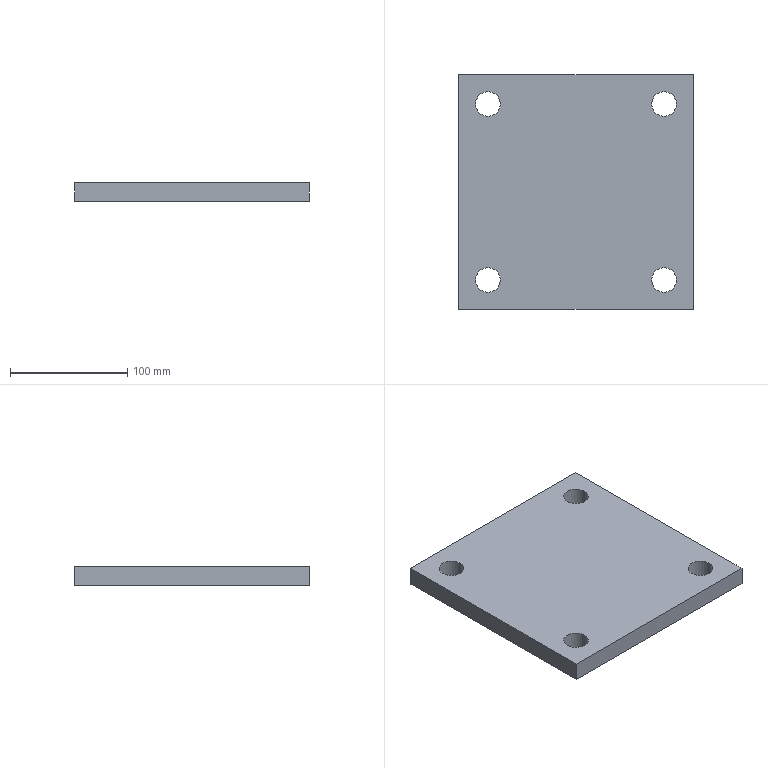Part | SolidWorks | features Extrusion 1, ICE 1, RefAxis 1 | 1 solid | 14 faces | box 200 x 200 x 16 mm | volume 617833 mm3 | cylinder 8 | plane 6 | commonest cylinder face diameters 21 x8
STEP:
#1=CARTESIAN_POINT('',(64.5,-75.,-8.));
#2=VERTEX_POINT('',#1);
#3=CARTESIAN_POINT('',(85.5,-75.,-8.));
#4=VERTEX_POINT('',#3);
#5=CARTESIAN_POINT('',(75.,-75.,-8.));
#6=DIRECTION('',(0.,0.,1.));
#7=DIRECTION('',(1.,0.,0.));
#8=AXIS2_PLACEMENT_3D('',#5,#6,#7);
#9=CIRCLE('',#8,10.5);
#10=EDGE_CURVE('',#2,#4,#9,.T.);
#11=ORIENTED_EDGE('',*,*,#10,.F.);
#12=CARTESIAN_POINT('',(64.5,-75.,8.));
#13=VERTEX_POINT('',#12);
#14=CARTESIAN_POINT('',(64.5,-75.,-8.));
#15=DIRECTION('',(0.,0.,1.));
#16=VECTOR('',#15,1000.);
#17=LINE('',#14,#16);
#18=EDGE_CURVE('',#2,#13,#17,.T.);
#19=ORIENTED_EDGE('',*,*,#18,.T.);
#20=CARTESIAN_POINT('',(85.5,-75.,8.));
#21=VERTEX_POINT('',#20);
#22=CARTESIAN_POINT('',(75.,-75.,8.));
#23=DIRECTION('',(0.,0.,1.));
#24=DIRECTION('',(1.,0.,0.));
#25=AXIS2_PLACEMENT_3D('',#22,#23,#24);
#26=CIRCLE('',#25,10.5);
#27=EDGE_CURVE('',#13,#21,#26,.T.);
#28=ORIENTED_EDGE('',*,*,#27,.T.);
#29=CARTESIAN_POINT('',(85.5,-75.,-8.));
#30=DIRECTION('',(0.,0.,1.));
#31=VECTOR('',#30,1000.);
#32=LINE('',#29,#31);
#33=EDGE_CURVE('',#4,#21,#32,.T.);
#34=ORIENTED_EDGE('',*,*,#33,.F.);
#35=EDGE_LOOP('',(#11,#19,#28,#34));
#36=FACE_OUTER_BOUND('',#35,.T.);
#37=CARTESIAN_POINT('',(75.,-75.,-8.));
#38=DIRECTION('',(0.,0.,1.));
#39=DIRECTION('',(1.,0.,0.));
#40=AXIS2_PLACEMENT_3D('',#37,#38,#39);
#41=CYLINDRICAL_SURFACE('',#40,10.5);
#42=ADVANCED_FACE('',(#36),#41,.F.);
#43=CARTESIAN_POINT('',(-85.5,-75.,-8.));
#44=VERTEX_POINT('',#43);
#45=CARTESIAN_POINT('',(-64.5,-75.,-8.));
#46=VERTEX_POINT('',#45);
#47=CARTESIAN_POINT('',(-75.,-75.,-8.));
#48=DIRECTION('',(0.,0.,1.));
#49=DIRECTION('',(1.,0.,0.));
#50=AXIS2_PLACEMENT_3D('',#47,#48,#49);
#51=CIRCLE('',#50,10.5);
#52=EDGE_CURVE('',#44,#46,#51,.T.);
#53=ORIENTED_EDGE('',*,*,#52,.F.);
#54=CARTESIAN_POINT('',(-85.5,-75.,8.));
#55=VERTEX_POINT('',#54);
#56=CARTESIAN_POINT('',(-85.5,-75.,-8.));
#57=DIRECTION('',(0.,0.,1.));
#58=VECTOR('',#57,1000.);
#59=LINE('',#56,#58);
#60=EDGE_CURVE('',#44,#55,#59,.T.);
#61=ORIENTED_EDGE('',*,*,#60,.T.);
#62=CARTESIAN_POINT('',(-64.5,-75.,8.));
#63=VERTEX_POINT('',#62);
#64=CARTESIAN_POINT('',(-75.,-75.,8.));
#65=DIRECTION('',(0.,0.,1.));
#66=DIRECTION('',(1.,0.,0.));
#67=AXIS2_PLACEMENT_3D('',#64,#65,#66);
#68=CIRCLE('',#67,10.5);
#69=EDGE_CURVE('',#55,#63,#68,.T.);
#70=ORIENTED_EDGE('',*,*,#69,.T.);
#71=CARTESIAN_POINT('',(-64.5,-75.,-8.));
#72=DIRECTION('',(0.,0.,1.));
#73=VECTOR('',#72,1000.);
#74=LINE('',#71,#73);
#75=EDGE_CURVE('',#46,#63,#74,.T.);
#76=ORIENTED_EDGE('',*,*,#75,.F.);
#77=EDGE_LOOP('',(#53,#61,#70,#76));
#78=FACE_OUTER_BOUND('',#77,.T.);
#79=CARTESIAN_POINT('',(-75.,-75.,-8.));
#80=DIRECTION('',(0.,0.,1.));
#81=DIRECTION('',(1.,0.,0.));
#82=AXIS2_PLACEMENT_3D('',#79,#80,#81);
#83=CYLINDRICAL_SURFACE('',#82,10.5);
#84=ADVANCED_FACE('',(#78),#83,.F.);
#85=CARTESIAN_POINT('',(64.5,75.,-8.));
#86=VERTEX_POINT('',#85);
#87=CARTESIAN_POINT('',(85.5,75.,-8.));
#88=VERTEX_POINT('',#87);
#89=CARTESIAN_POINT('',(75.,75.,-8.));
#90=DIRECTION('',(0.,0.,1.));
#91=DIRECTION('',(1.,0.,0.));
#92=AXIS2_PLACEMENT_3D('',#89,#90,#91);
#93=CIRCLE('',#92,10.5);
#94=EDGE_CURVE('',#86,#88,#93,.T.);
#95=ORIENTED_EDGE('',*,*,#94,.F.);
#96=CARTESIAN_POINT('',(64.5,75.,8.));
#97=VERTEX_POINT('',#96);
#98=CARTESIAN_POINT('',(64.5,75.,-8.));
#99=DIRECTION('',(0.,0.,1.));
#100=VECTOR('',#99,1000.);
#101=LINE('',#98,#100);
#102=EDGE_CURVE('',#86,#97,#101,.T.);
#103=ORIENTED_EDGE('',*,*,#102,.T.);
#104=CARTESIAN_POINT('',(85.5,75.,8.));
#105=VERTEX_POINT('',#104);
#106=CARTESIAN_POINT('',(75.,75.,8.));
#107=DIRECTION('',(0.,0.,1.));
#108=DIRECTION('',(1.,0.,0.));
#109=AXIS2_PLACEMENT_3D('',#106,#107,#108);
#110=CIRCLE('',#109,10.5);
#111=EDGE_CURVE('',#97,#105,#110,.T.);
#112=ORIENTED_EDGE('',*,*,#111,.T.);
#113=CARTESIAN_POINT('',(85.5,75.,-8.));
#114=DIRECTION('',(0.,0.,1.));
#115=VECTOR('',#114,1000.);
#116=LINE('',#113,#115);
#117=EDGE_CURVE('',#88,#105,#116,.T.);
#118=ORIENTED_EDGE('',*,*,#117,.F.);
#119=EDGE_LOOP('',(#95,#103,#112,#118));
#120=FACE_OUTER_BOUND('',#119,.T.);
#121=CARTESIAN_POINT('',(75.,75.,-8.));
#122=DIRECTION('',(0.,0.,1.));
#123=DIRECTION('',(1.,0.,0.));
#124=AXIS2_PLACEMENT_3D('',#121,#122,#123);
#125=CYLINDRICAL_SURFACE('',#124,10.5);
#126=ADVANCED_FACE('',(#120),#125,.F.);
#127=CARTESIAN_POINT('',(-85.5,75.,-8.));
#128=VERTEX_POINT('',#127);
#129=CARTESIAN_POINT('',(-64.5,75.,-8.));
#130=VERTEX_POINT('',#129);
#131=CARTESIAN_POINT('',(-75.,75.,-8.));
#132=DIRECTION('',(0.,0.,1.));
#133=DIRECTION('',(1.,0.,0.));
#134=AXIS2_PLACEMENT_3D('',#131,#132,#133);
#135=CIRCLE('',#134,10.5);
#136=EDGE_CURVE('',#128,#130,#135,.T.);
#137=ORIENTED_EDGE('',*,*,#136,.F.);
#138=CARTESIAN_POINT('',(-85.5,75.,8.));
#139=VERTEX_POINT('',#138);
#140=CARTESIAN_POINT('',(-85.5,75.,-8.));
#141=DIRECTION('',(0.,0.,1.));
#142=VECTOR('',#141,1000.);
#143=LINE('',#140,#142);
#144=EDGE_CURVE('',#128,#139,#143,.T.);
#145=ORIENTED_EDGE('',*,*,#144,.T.);
#146=CARTESIAN_POINT('',(-64.5,75.,8.));
#147=VERTEX_POINT('',#146);
#148=CARTESIAN_POINT('',(-75.,75.,8.));
#149=DIRECTION('',(0.,0.,1.));
#150=DIRECTION('',(1.,0.,0.));
#151=AXIS2_PLACEMENT_3D('',#148,#149,#150);
#152=CIRCLE('',#151,10.5);
#153=EDGE_CURVE('',#139,#147,#152,.T.);
#154=ORIENTED_EDGE('',*,*,#153,.T.);
#155=CARTESIAN_POINT('',(-64.5,75.,-8.));
#156=DIRECTION('',(0.,0.,1.));
#157=VECTOR('',#156,1000.);
#158=LINE('',#155,#157);
#159=EDGE_CURVE('',#130,#147,#158,.T.);
#160=ORIENTED_EDGE('',*,*,#159,.F.);
#161=EDGE_LOOP('',(#137,#145,#154,#160));
#162=FACE_OUTER_BOUND('',#161,.T.);
#163=CARTESIAN_POINT('',(-75.,75.,-8.));
#164=DIRECTION('',(0.,0.,1.));
#165=DIRECTION('',(1.,0.,0.));
#166=AXIS2_PLACEMENT_3D('',#163,#164,#165);
#167=CYLINDRICAL_SURFACE('',#166,10.5);
#168=ADVANCED_FACE('',(#162),#167,.F.);
#169=CARTESIAN_POINT('',(-100.,100.,-8.));
#170=VERTEX_POINT('',#169);
#171=CARTESIAN_POINT('',(-100.,-100.,-8.));
#172=VERTEX_POINT('',#171);
#173=CARTESIAN_POINT('',(-100.,-100.,-8.));
#174=DIRECTION('',(0.,-1.,0.));
#175=VECTOR('',#174,1000.);
#176=LINE('',#173,#175);
#177=EDGE_CURVE('',#170,#172,#176,.T.);
#178=ORIENTED_EDGE('',*,*,#177,.T.);
#179=CARTESIAN_POINT('',(-100.,-100.,8.));
#180=VERTEX_POINT('',#179);
#181=CARTESIAN_POINT('',(-100.,-100.,8.));
#182=DIRECTION('',(0.,0.,-1.));
#183=VECTOR('',#182,1000.);
#184=LINE('',#181,#183);
#185=EDGE_CURVE('',#180,#172,#184,.T.);
#186=ORIENTED_EDGE('',*,*,#185,.F.);
#187=CARTESIAN_POINT('',(-100.,100.,8.));
#188=VERTEX_POINT('',#187);
#189=CARTESIAN_POINT('',(-100.,-100.,8.));
#190=DIRECTION('',(0.,-1.,0.));
#191=VECTOR('',#190,1000.);
#192=LINE('',#189,#191);
#193=EDGE_CURVE('',#188,#180,#192,.T.);
#194=ORIENTED_EDGE('',*,*,#193,.F.);
#195=CARTESIAN_POINT('',(-100.,100.,8.));
#196=DIRECTION('',(0.,0.,-1.));
#197=VECTOR('',#196,1000.);
#198=LINE('',#195,#197);
#199=EDGE_CURVE('',#188,#170,#198,.T.);
#200=ORIENTED_EDGE('',*,*,#199,.T.);
#201=EDGE_LOOP('',(#178,#186,#194,#200));
#202=FACE_OUTER_BOUND('',#201,.T.);
#203=CARTESIAN_POINT('',(-100.,-100.,8.));
#204=DIRECTION('',(1.,0.,0.));
#205=DIRECTION('',(0.,1.,0.));
#206=AXIS2_PLACEMENT_3D('',#203,#204,#205);
#207=PLANE('',#206);
#208=ADVANCED_FACE('',(#202),#207,.F.);
#209=CARTESIAN_POINT('',(100.,-100.,-8.));
#210=VERTEX_POINT('',#209);
#211=CARTESIAN_POINT('',(100.,-100.,-8.));
#212=DIRECTION('',(1.,0.,0.));
#213=VECTOR('',#212,1000.);
#214=LINE('',#211,#213);
#215=EDGE_CURVE('',#172,#210,#214,.T.);
#216=ORIENTED_EDGE('',*,*,#215,.T.);
#217=CARTESIAN_POINT('',(100.,-100.,8.));
#218=VERTEX_POINT('',#217);
#219=CARTESIAN_POINT('',(100.,-100.,8.));
#220=DIRECTION('',(0.,0.,-1.));
#221=VECTOR('',#220,1000.);
#222=LINE('',#219,#221);
#223=EDGE_CURVE('',#218,#210,#222,.T.);
#224=ORIENTED_EDGE('',*,*,#223,.F.);
#225=CARTESIAN_POINT('',(100.,-100.,8.));
#226=DIRECTION('',(1.,0.,0.));
#227=VECTOR('',#226,1000.);
#228=LINE('',#225,#227);
#229=EDGE_CURVE('',#180,#218,#228,.T.);
#230=ORIENTED_EDGE('',*,*,#229,.F.);
#231=ORIENTED_EDGE('',*,*,#185,.T.);
#232=EDGE_LOOP('',(#216,#224,#230,#231));
#233=FACE_OUTER_BOUND('',#232,.T.);
#234=CARTESIAN_POINT('',(100.,-100.,8.));
#235=DIRECTION('',(0.,1.,0.));
#236=DIRECTION('',(-1.,0.,0.));
#237=AXIS2_PLACEMENT_3D('',#234,#235,#236);
#238=PLANE('',#237);
#239=ADVANCED_FACE('',(#233),#238,.F.);
#240=CARTESIAN_POINT('',(100.,100.,-8.));
#241=VERTEX_POINT('',#240);
#242=CARTESIAN_POINT('',(100.,100.,-8.));
#243=DIRECTION('',(0.,1.,0.));
#244=VECTOR('',#243,1000.);
#245=LINE('',#242,#244);
#246=EDGE_CURVE('',#210,#241,#245,.T.);
#247=ORIENTED_EDGE('',*,*,#246,.T.);
#248=CARTESIAN_POINT('',(100.,100.,8.));
#249=VERTEX_POINT('',#248);
#250=CARTESIAN_POINT('',(100.,100.,8.));
#251=DIRECTION('',(0.,0.,-1.));
#252=VECTOR('',#251,1000.);
#253=LINE('',#250,#252);
#254=EDGE_CURVE('',#249,#241,#253,.T.);
#255=ORIENTED_EDGE('',*,*,#254,.F.);
#256=CARTESIAN_POINT('',(100.,100.,8.));
#257=DIRECTION('',(0.,1.,0.));
#258=VECTOR('',#257,1000.);
#259=LINE('',#256,#258);
#260=EDGE_CURVE('',#218,#249,#259,.T.);
#261=ORIENTED_EDGE('',*,*,#260,.F.);
#262=ORIENTED_EDGE('',*,*,#223,.T.);
#263=EDGE_LOOP('',(#247,#255,#261,#262));
#264=FACE_OUTER_BOUND('',#263,.T.);
#265=CARTESIAN_POINT('',(100.,100.,8.));
#266=DIRECTION('',(-1.,0.,0.));
#267=DIRECTION('',(0.,-1.,0.));
#268=AXIS2_PLACEMENT_3D('',#265,#266,#267);
#269=PLANE('',#268);
#270=ADVANCED_FACE('',(#264),#269,.F.);
#271=CARTESIAN_POINT('',(-100.,100.,-8.));
#272=DIRECTION('',(-1.,0.,0.));
#273=VECTOR('',#272,1000.);
#274=LINE('',#271,#273);
#275=EDGE_CURVE('',#241,#170,#274,.T.);
#276=ORIENTED_EDGE('',*,*,#275,.T.);
#277=ORIENTED_EDGE('',*,*,#199,.F.);
#278=CARTESIAN_POINT('',(-100.,100.,8.));
#279=DIRECTION('',(-1.,0.,0.));
#280=VECTOR('',#279,1000.);
#281=LINE('',#278,#280);
#282=EDGE_CURVE('',#249,#188,#281,.T.);
#283=ORIENTED_EDGE('',*,*,#282,.F.);
#284=ORIENTED_EDGE('',*,*,#254,.T.);
#285=EDGE_LOOP('',(#276,#277,#283,#284));
#286=FACE_OUTER_BOUND('',#285,.T.);
#287=CARTESIAN_POINT('',(-100.,100.,8.));
#288=DIRECTION('',(0.,-1.,0.));
#289=DIRECTION('',(0.,0.,-1.));
#290=AXIS2_PLACEMENT_3D('',#287,#288,#289);
#291=PLANE('',#290);
#292=ADVANCED_FACE('',(#286),#291,.F.);
#293=CARTESIAN_POINT('',(75.,-75.,8.));
#294=DIRECTION('',(0.,0.,1.));
#295=DIRECTION('',(1.,0.,0.));
#296=AXIS2_PLACEMENT_3D('',#293,#294,#295);
#297=CIRCLE('',#296,10.5);
#298=EDGE_CURVE('',#21,#13,#297,.T.);
#299=ORIENTED_EDGE('',*,*,#298,.F.);
#300=ORIENTED_EDGE('',*,*,#27,.F.);
#301=EDGE_LOOP('',(#299,#300));
#302=FACE_BOUND('',#301,.T.);
#303=CARTESIAN_POINT('',(-75.,-75.,8.));
#304=DIRECTION('',(0.,0.,1.));
#305=DIRECTION('',(1.,0.,0.));
#306=AXIS2_PLACEMENT_3D('',#303,#304,#305);
#307=CIRCLE('',#306,10.5);
#308=EDGE_CURVE('',#63,#55,#307,.T.);
#309=ORIENTED_EDGE('',*,*,#308,.F.);
#310=ORIENTED_EDGE('',*,*,#69,.F.);
#311=EDGE_LOOP('',(#309,#310));
#312=FACE_BOUND('',#311,.T.);
#313=CARTESIAN_POINT('',(75.,75.,8.));
#314=DIRECTION('',(0.,0.,1.));
#315=DIRECTION('',(1.,0.,0.));
#316=AXIS2_PLACEMENT_3D('',#313,#314,#315);
#317=CIRCLE('',#316,10.5);
#318=EDGE_CURVE('',#105,#97,#317,.T.);
#319=ORIENTED_EDGE('',*,*,#318,.F.);
#320=ORIENTED_EDGE('',*,*,#111,.F.);
#321=EDGE_LOOP('',(#319,#320));
#322=FACE_BOUND('',#321,.T.);
#323=CARTESIAN_POINT('',(-75.,75.,8.));
#324=DIRECTION('',(0.,0.,1.));
#325=DIRECTION('',(1.,0.,0.));
#326=AXIS2_PLACEMENT_3D('',#323,#324,#325);
#327=CIRCLE('',#326,10.5);
#328=EDGE_CURVE('',#147,#139,#327,.T.);
#329=ORIENTED_EDGE('',*,*,#328,.F.);
#330=ORIENTED_EDGE('',*,*,#153,.F.);
#331=EDGE_LOOP('',(#329,#330));
#332=FACE_BOUND('',#331,.T.);
#333=ORIENTED_EDGE('',*,*,#193,.T.);
#334=ORIENTED_EDGE('',*,*,#229,.T.);
#335=ORIENTED_EDGE('',*,*,#260,.T.);
#336=ORIENTED_EDGE('',*,*,#282,.T.);
#337=EDGE_LOOP('',(#333,#334,#335,#336));
#338=FACE_OUTER_BOUND('',#337,.T.);
#339=CARTESIAN_POINT('',(-100.,100.,8.));
#340=DIRECTION('',(0.,0.,-1.));
#341=DIRECTION('',(-1.,0.,0.));
#342=AXIS2_PLACEMENT_3D('',#339,#340,#341);
#343=PLANE('',#342);
#344=ADVANCED_FACE('',(#302,#312,#322,#332,#338),#343,.F.);
#345=CARTESIAN_POINT('',(75.,-75.,-8.));
#346=DIRECTION('',(0.,0.,1.));
#347=DIRECTION('',(1.,0.,0.));
#348=AXIS2_PLACEMENT_3D('',#345,#346,#347);
#349=CIRCLE('',#348,10.5);
#350=EDGE_CURVE('',#4,#2,#349,.T.);
#351=ORIENTED_EDGE('',*,*,#350,.T.);
#352=ORIENTED_EDGE('',*,*,#10,.T.);
#353=EDGE_LOOP('',(#351,#352));
#354=FACE_BOUND('',#353,.T.);
#355=CARTESIAN_POINT('',(-75.,-75.,-8.));
#356=DIRECTION('',(0.,0.,1.));
#357=DIRECTION('',(1.,0.,0.));
#358=AXIS2_PLACEMENT_3D('',#355,#356,#357);
#359=CIRCLE('',#358,10.5);
#360=EDGE_CURVE('',#46,#44,#359,.T.);
#361=ORIENTED_EDGE('',*,*,#360,.T.);
#362=ORIENTED_EDGE('',*,*,#52,.T.);
#363=EDGE_LOOP('',(#361,#362));
#364=FACE_BOUND('',#363,.T.);
#365=CARTESIAN_POINT('',(75.,75.,-8.));
#366=DIRECTION('',(0.,0.,1.));
#367=DIRECTION('',(1.,0.,0.));
#368=AXIS2_PLACEMENT_3D('',#365,#366,#367);
#369=CIRCLE('',#368,10.5);
#370=EDGE_CURVE('',#88,#86,#369,.T.);
#371=ORIENTED_EDGE('',*,*,#370,.T.);
#372=ORIENTED_EDGE('',*,*,#94,.T.);
#373=EDGE_LOOP('',(#371,#372));
#374=FACE_BOUND('',#373,.T.);
#375=CARTESIAN_POINT('',(-75.,75.,-8.));
#376=DIRECTION('',(0.,0.,1.));
#377=DIRECTION('',(1.,0.,0.));
#378=AXIS2_PLACEMENT_3D('',#375,#376,#377);
#379=CIRCLE('',#378,10.5);
#380=EDGE_CURVE('',#130,#128,#379,.T.);
#381=ORIENTED_EDGE('',*,*,#380,.T.);
#382=ORIENTED_EDGE('',*,*,#136,.T.);
#383=EDGE_LOOP('',(#381,#382));
#384=FACE_BOUND('',#383,.T.);
#385=ORIENTED_EDGE('',*,*,#177,.F.);
#386=ORIENTED_EDGE('',*,*,#275,.F.);
#387=ORIENTED_EDGE('',*,*,#246,.F.);
#388=ORIENTED_EDGE('',*,*,#215,.F.);
#389=EDGE_LOOP('',(#385,#386,#387,#388));
#390=FACE_OUTER_BOUND('',#389,.T.);
#391=CARTESIAN_POINT('',(-100.,100.,-8.));
#392=DIRECTION('',(0.,0.,-1.));
#393=DIRECTION('',(-1.,0.,0.));
#394=AXIS2_PLACEMENT_3D('',#391,#392,#393);
#395=PLANE('',#394);
#396=ADVANCED_FACE('',(#354,#364,#374,#384,#390),#395,.T.);
#397=ORIENTED_EDGE('',*,*,#144,.F.);
#398=ORIENTED_EDGE('',*,*,#380,.F.);
#399=ORIENTED_EDGE('',*,*,#159,.T.);
#400=ORIENTED_EDGE('',*,*,#328,.T.);
#401=EDGE_LOOP('',(#397,#398,#399,#400));
#402=FACE_OUTER_BOUND('',#401,.T.);
#403=CARTESIAN_POINT('',(-75.,75.,-8.));
#404=DIRECTION('',(0.,0.,1.));
#405=DIRECTION('',(1.,0.,0.));
#406=AXIS2_PLACEMENT_3D('',#403,#404,#405);
#407=CYLINDRICAL_SURFACE('',#406,10.5);
#408=ADVANCED_FACE('',(#402),#407,.F.);
#409=ORIENTED_EDGE('',*,*,#102,.F.);
#410=ORIENTED_EDGE('',*,*,#370,.F.);
#411=ORIENTED_EDGE('',*,*,#117,.T.);
#412=ORIENTED_EDGE('',*,*,#318,.T.);
#413=EDGE_LOOP('',(#409,#410,#411,#412));
#414=FACE_OUTER_BOUND('',#413,.T.);
#415=CARTESIAN_POINT('',(75.,75.,-8.));
#416=DIRECTION('',(0.,0.,1.));
#417=DIRECTION('',(1.,0.,0.));
#418=AXIS2_PLACEMENT_3D('',#415,#416,#417);
#419=CYLINDRICAL_SURFACE('',#418,10.5);
#420=ADVANCED_FACE('',(#414),#419,.F.);
#421=ORIENTED_EDGE('',*,*,#60,.F.);
#422=ORIENTED_EDGE('',*,*,#360,.F.);
#423=ORIENTED_EDGE('',*,*,#75,.T.);
#424=ORIENTED_EDGE('',*,*,#308,.T.);
#425=EDGE_LOOP('',(#421,#422,#423,#424));
#426=FACE_OUTER_BOUND('',#425,.T.);
#427=CARTESIAN_POINT('',(-75.,-75.,-8.));
#428=DIRECTION('',(0.,0.,1.));
#429=DIRECTION('',(1.,0.,0.));
#430=AXIS2_PLACEMENT_3D('',#427,#428,#429);
#431=CYLINDRICAL_SURFACE('',#430,10.5);
#432=ADVANCED_FACE('',(#426),#431,.F.);
#433=ORIENTED_EDGE('',*,*,#18,.F.);
#434=ORIENTED_EDGE('',*,*,#350,.F.);
#435=ORIENTED_EDGE('',*,*,#33,.T.);
#436=ORIENTED_EDGE('',*,*,#298,.T.);
#437=EDGE_LOOP('',(#433,#434,#435,#436));
#438=FACE_OUTER_BOUND('',#437,.T.);
#439=CARTESIAN_POINT('',(75.,-75.,-8.));
#440=DIRECTION('',(0.,0.,1.));
#441=DIRECTION('',(1.,0.,0.));
#442=AXIS2_PLACEMENT_3D('',#439,#440,#441);
#443=CYLINDRICAL_SURFACE('',#442,10.5);
#444=ADVANCED_FACE('',(#438),#443,.F.);
#445=CLOSED_SHELL('',(#42,#84,#126,#168,#208,#239,#270,#292,#344,#396,#408,#420,#432,#444));
#446=MANIFOLD_SOLID_BREP('',#445);
#447=CARTESIAN_POINT('',(0.,0.,0.));
#448=DIRECTION('',(0.,0.,1.));
#449=DIRECTION('',(1.,0.,0.));
#450=AXIS2_PLACEMENT_3D('',#447,#448,#449);
#451=(LENGTH_UNIT()NAMED_UNIT(*)SI_UNIT(.MILLI.,.METRE.));
#452=UNCERTAINTY_MEASURE_WITH_UNIT(LENGTH_MEASURE(0.00001),#451,'','');
#453=(NAMED_UNIT(*)PLANE_ANGLE_UNIT()SI_UNIT($,.RADIAN.));
#454=(NAMED_UNIT(*)SI_UNIT($,.STERADIAN.)SOLID_ANGLE_UNIT());
#455=(GEOMETRIC_REPRESENTATION_CONTEXT(3)GLOBAL_UNCERTAINTY_ASSIGNED_CONTEXT((#452))GLOBAL_UNIT_ASSIGNED_CONTEXT((#451,#453,#454))REPRESENTATION_CONTEXT('',''));
#456=ADVANCED_BREP_SHAPE_REPRESENTATION('',(#446,#450),#455);